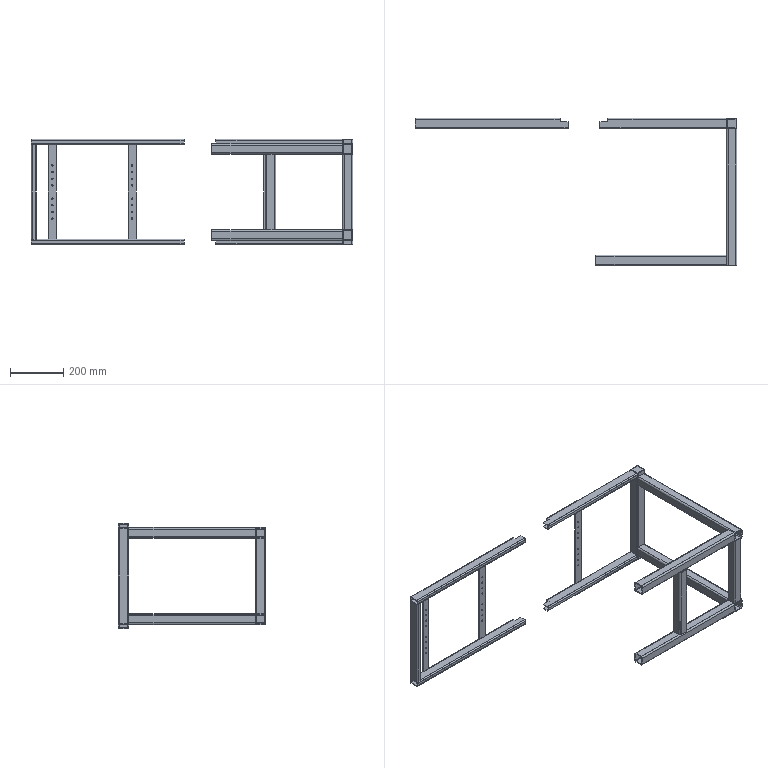Part | SolidWorks | features ICE 3, WeldMemberFeat 3, WeldCornerFeat 2, 3DProfileFeature 1, EndCap 1, HoleWzd 1, WeldmentFeature 1 | 17 solids | 322 faces | box 1210 x 555 x 396 mm | volume 2067194 mm3 | plane 162 | cylinder 160 | commonest cylinder face diameters 5 x84 6.4 x24 12.8 x24 10 x20 4.6 x4 9.2 x4